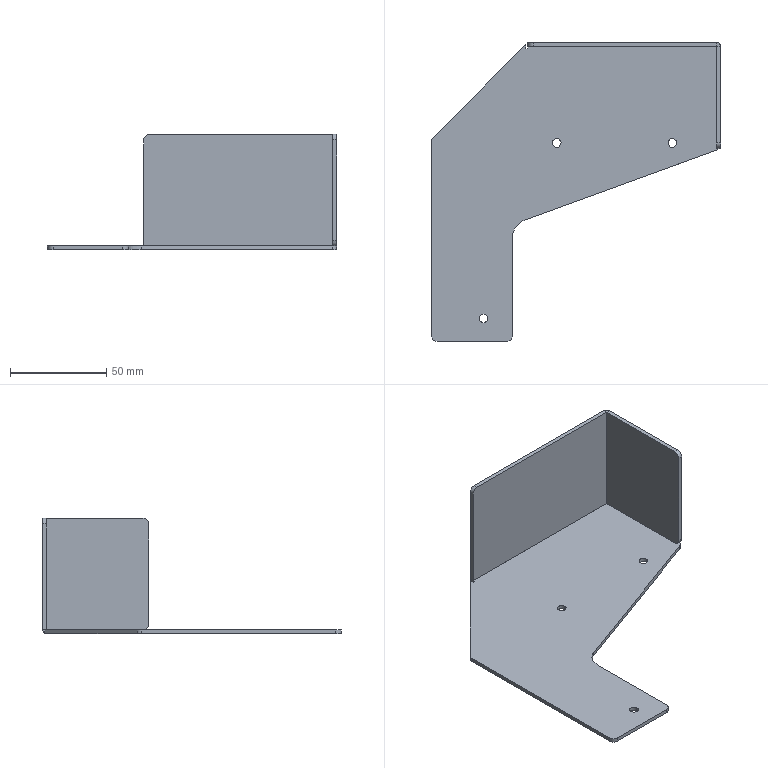Part | STEP file | 1 solid | 43 faces | box 150 x 155 x 60 mm | volume 44145 mm3 | plane 25 | cylinder 18 | commonest cylinder face diameters 6 x7 4.5 x6 0.02 x2 4.02 x2 20 x1